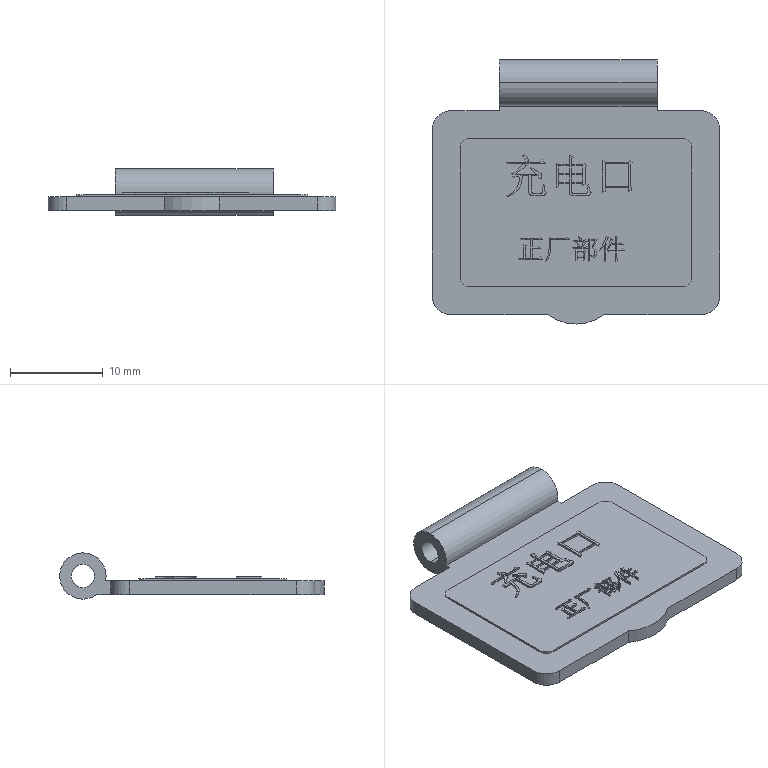Part | SolidWorks | features BaseBody 1 | 1 solid | 283 faces | box 31 x 28.5 x 5 mm | volume 1380 mm3 | plane 206 | spline 63 | cylinder 14 | commonest cylinder face diameters 2 x4 4 x4 5 x3 2.5 x2 10 x1